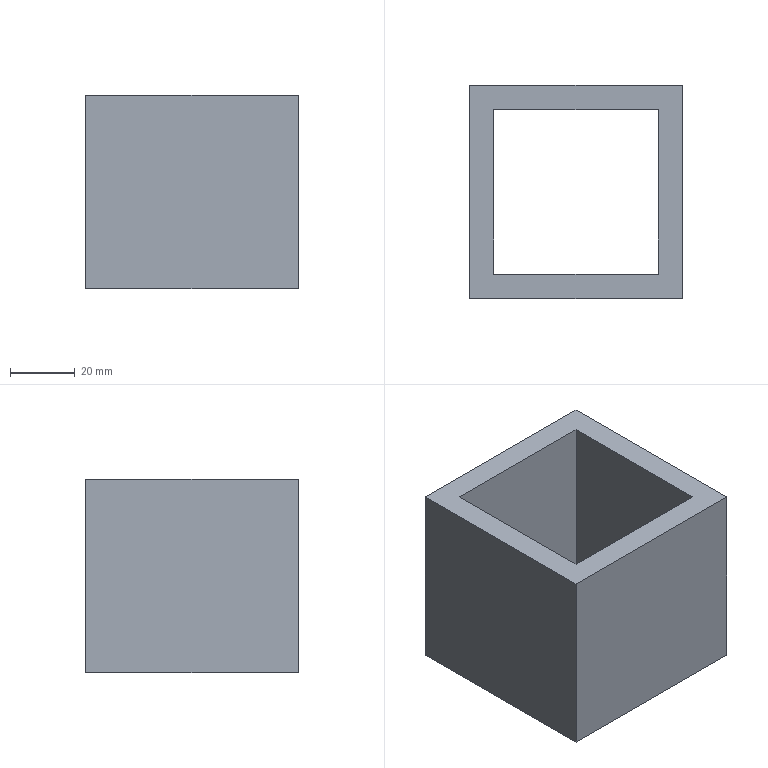Part | SolidWorks | features Extrusion 1 | 1 solid | 10 faces | box 66 x 66 x 60 mm | volume 105300 mm3 | plane 10
STEP:
#1=CARTESIAN_POINT('',(-33.,33.,30.));
#2=VERTEX_POINT('',#1);
#3=CARTESIAN_POINT('',(-33.,-33.,30.));
#4=VERTEX_POINT('',#3);
#5=CARTESIAN_POINT('',(-33.,33.,30.));
#6=DIRECTION('',(0.,-1.,0.));
#7=VECTOR('',#6,1000.);
#8=LINE('',#5,#7);
#9=EDGE_CURVE('',#2,#4,#8,.T.);
#10=ORIENTED_EDGE('',*,*,#9,.F.);
#11=CARTESIAN_POINT('',(-33.,33.,-30.));
#12=VERTEX_POINT('',#11);
#13=CARTESIAN_POINT('',(-33.,33.,-30.));
#14=DIRECTION('',(0.,0.,1.));
#15=VECTOR('',#14,1000.);
#16=LINE('',#13,#15);
#17=EDGE_CURVE('',#12,#2,#16,.T.);
#18=ORIENTED_EDGE('',*,*,#17,.F.);
#19=CARTESIAN_POINT('',(-33.,-33.,-30.));
#20=VERTEX_POINT('',#19);
#21=CARTESIAN_POINT('',(-33.,33.,-30.));
#22=DIRECTION('',(0.,-1.,0.));
#23=VECTOR('',#22,1000.);
#24=LINE('',#21,#23);
#25=EDGE_CURVE('',#12,#20,#24,.T.);
#26=ORIENTED_EDGE('',*,*,#25,.T.);
#27=CARTESIAN_POINT('',(-33.,-33.,-30.));
#28=DIRECTION('',(0.,0.,1.));
#29=VECTOR('',#28,1000.);
#30=LINE('',#27,#29);
#31=EDGE_CURVE('',#20,#4,#30,.T.);
#32=ORIENTED_EDGE('',*,*,#31,.T.);
#33=EDGE_LOOP('',(#10,#18,#26,#32));
#34=FACE_OUTER_BOUND('',#33,.T.);
#35=CARTESIAN_POINT('',(-33.,33.,-30.));
#36=DIRECTION('',(-1.,0.,0.));
#37=DIRECTION('',(0.,0.,1.));
#38=AXIS2_PLACEMENT_3D('',#35,#36,#37);
#39=PLANE('',#38);
#40=ADVANCED_FACE('',(#34),#39,.T.);
#41=CARTESIAN_POINT('',(33.,33.,30.));
#42=VERTEX_POINT('',#41);
#43=CARTESIAN_POINT('',(33.,33.,30.));
#44=DIRECTION('',(-1.,0.,0.));
#45=VECTOR('',#44,1000.);
#46=LINE('',#43,#45);
#47=EDGE_CURVE('',#42,#2,#46,.T.);
#48=ORIENTED_EDGE('',*,*,#47,.F.);
#49=CARTESIAN_POINT('',(33.,33.,-30.));
#50=VERTEX_POINT('',#49);
#51=CARTESIAN_POINT('',(33.,33.,-30.));
#52=DIRECTION('',(0.,0.,1.));
#53=VECTOR('',#52,1000.);
#54=LINE('',#51,#53);
#55=EDGE_CURVE('',#50,#42,#54,.T.);
#56=ORIENTED_EDGE('',*,*,#55,.F.);
#57=CARTESIAN_POINT('',(33.,33.,-30.));
#58=DIRECTION('',(-1.,0.,0.));
#59=VECTOR('',#58,1000.);
#60=LINE('',#57,#59);
#61=EDGE_CURVE('',#50,#12,#60,.T.);
#62=ORIENTED_EDGE('',*,*,#61,.T.);
#63=ORIENTED_EDGE('',*,*,#17,.T.);
#64=EDGE_LOOP('',(#48,#56,#62,#63));
#65=FACE_OUTER_BOUND('',#64,.T.);
#66=CARTESIAN_POINT('',(33.,33.,-30.));
#67=DIRECTION('',(0.,1.,0.));
#68=DIRECTION('',(0.,0.,1.));
#69=AXIS2_PLACEMENT_3D('',#66,#67,#68);
#70=PLANE('',#69);
#71=ADVANCED_FACE('',(#65),#70,.T.);
#72=CARTESIAN_POINT('',(33.,-33.,30.));
#73=VERTEX_POINT('',#72);
#74=CARTESIAN_POINT('',(33.,-33.,30.));
#75=DIRECTION('',(0.,1.,0.));
#76=VECTOR('',#75,1000.);
#77=LINE('',#74,#76);
#78=EDGE_CURVE('',#73,#42,#77,.T.);
#79=ORIENTED_EDGE('',*,*,#78,.F.);
#80=CARTESIAN_POINT('',(33.,-33.,-30.));
#81=VERTEX_POINT('',#80);
#82=CARTESIAN_POINT('',(33.,-33.,-30.));
#83=DIRECTION('',(0.,0.,1.));
#84=VECTOR('',#83,1000.);
#85=LINE('',#82,#84);
#86=EDGE_CURVE('',#81,#73,#85,.T.);
#87=ORIENTED_EDGE('',*,*,#86,.F.);
#88=CARTESIAN_POINT('',(33.,-33.,-30.));
#89=DIRECTION('',(0.,1.,0.));
#90=VECTOR('',#89,1000.);
#91=LINE('',#88,#90);
#92=EDGE_CURVE('',#81,#50,#91,.T.);
#93=ORIENTED_EDGE('',*,*,#92,.T.);
#94=ORIENTED_EDGE('',*,*,#55,.T.);
#95=EDGE_LOOP('',(#79,#87,#93,#94));
#96=FACE_OUTER_BOUND('',#95,.T.);
#97=CARTESIAN_POINT('',(33.,-33.,-30.));
#98=DIRECTION('',(1.,0.,0.));
#99=DIRECTION('',(0.,0.,-1.));
#100=AXIS2_PLACEMENT_3D('',#97,#98,#99);
#101=PLANE('',#100);
#102=ADVANCED_FACE('',(#96),#101,.T.);
#103=CARTESIAN_POINT('',(-33.,-33.,30.));
#104=DIRECTION('',(1.,0.,0.));
#105=VECTOR('',#104,1000.);
#106=LINE('',#103,#105);
#107=EDGE_CURVE('',#4,#73,#106,.T.);
#108=ORIENTED_EDGE('',*,*,#107,.F.);
#109=ORIENTED_EDGE('',*,*,#31,.F.);
#110=CARTESIAN_POINT('',(-33.,-33.,-30.));
#111=DIRECTION('',(1.,0.,0.));
#112=VECTOR('',#111,1000.);
#113=LINE('',#110,#112);
#114=EDGE_CURVE('',#20,#81,#113,.T.);
#115=ORIENTED_EDGE('',*,*,#114,.T.);
#116=ORIENTED_EDGE('',*,*,#86,.T.);
#117=EDGE_LOOP('',(#108,#109,#115,#116));
#118=FACE_OUTER_BOUND('',#117,.T.);
#119=CARTESIAN_POINT('',(-33.,-33.,-30.));
#120=DIRECTION('',(0.,-1.,0.));
#121=DIRECTION('',(0.,0.,-1.));
#122=AXIS2_PLACEMENT_3D('',#119,#120,#121);
#123=PLANE('',#122);
#124=ADVANCED_FACE('',(#118),#123,.T.);
#125=CARTESIAN_POINT('',(25.5,25.5,-30.));
#126=VERTEX_POINT('',#125);
#127=CARTESIAN_POINT('',(-25.5,25.5,-30.));
#128=VERTEX_POINT('',#127);
#129=CARTESIAN_POINT('',(25.5,25.5,-30.));
#130=DIRECTION('',(-1.,0.,0.));
#131=VECTOR('',#130,1000.);
#132=LINE('',#129,#131);
#133=EDGE_CURVE('',#126,#128,#132,.T.);
#134=ORIENTED_EDGE('',*,*,#133,.T.);
#135=CARTESIAN_POINT('',(-25.5,-25.5,-30.));
#136=VERTEX_POINT('',#135);
#137=CARTESIAN_POINT('',(-25.5,25.5,-30.));
#138=DIRECTION('',(0.,-1.,0.));
#139=VECTOR('',#138,1000.);
#140=LINE('',#137,#139);
#141=EDGE_CURVE('',#128,#136,#140,.T.);
#142=ORIENTED_EDGE('',*,*,#141,.T.);
#143=CARTESIAN_POINT('',(25.5,-25.5,-30.));
#144=VERTEX_POINT('',#143);
#145=CARTESIAN_POINT('',(-25.5,-25.5,-30.));
#146=DIRECTION('',(1.,0.,0.));
#147=VECTOR('',#146,1000.);
#148=LINE('',#145,#147);
#149=EDGE_CURVE('',#136,#144,#148,.T.);
#150=ORIENTED_EDGE('',*,*,#149,.T.);
#151=CARTESIAN_POINT('',(25.5,-25.5,-30.));
#152=DIRECTION('',(0.,1.,0.));
#153=VECTOR('',#152,1000.);
#154=LINE('',#151,#153);
#155=EDGE_CURVE('',#144,#126,#154,.T.);
#156=ORIENTED_EDGE('',*,*,#155,.T.);
#157=EDGE_LOOP('',(#134,#142,#150,#156));
#158=FACE_BOUND('',#157,.T.);
#159=ORIENTED_EDGE('',*,*,#25,.F.);
#160=ORIENTED_EDGE('',*,*,#61,.F.);
#161=ORIENTED_EDGE('',*,*,#92,.F.);
#162=ORIENTED_EDGE('',*,*,#114,.F.);
#163=EDGE_LOOP('',(#159,#160,#161,#162));
#164=FACE_OUTER_BOUND('',#163,.T.);
#165=CARTESIAN_POINT('',(0.,0.,-30.));
#166=DIRECTION('',(0.,0.,1.));
#167=DIRECTION('',(1.,0.,0.));
#168=AXIS2_PLACEMENT_3D('',#165,#166,#167);
#169=PLANE('',#168);
#170=ADVANCED_FACE('',(#158,#164),#169,.F.);
#171=CARTESIAN_POINT('',(-25.5,25.5,30.));
#172=VERTEX_POINT('',#171);
#173=CARTESIAN_POINT('',(-25.5,-25.5,30.));
#174=VERTEX_POINT('',#173);
#175=CARTESIAN_POINT('',(-25.5,25.5,30.));
#176=DIRECTION('',(0.,-1.,0.));
#177=VECTOR('',#176,1000.);
#178=LINE('',#175,#177);
#179=EDGE_CURVE('',#172,#174,#178,.T.);
#180=ORIENTED_EDGE('',*,*,#179,.F.);
#181=CARTESIAN_POINT('',(25.5,25.5,30.));
#182=VERTEX_POINT('',#181);
#183=CARTESIAN_POINT('',(25.5,25.5,30.));
#184=DIRECTION('',(-1.,0.,0.));
#185=VECTOR('',#184,1000.);
#186=LINE('',#183,#185);
#187=EDGE_CURVE('',#182,#172,#186,.T.);
#188=ORIENTED_EDGE('',*,*,#187,.F.);
#189=CARTESIAN_POINT('',(25.5,-25.5,30.));
#190=VERTEX_POINT('',#189);
#191=CARTESIAN_POINT('',(25.5,-25.5,30.));
#192=DIRECTION('',(0.,1.,0.));
#193=VECTOR('',#192,1000.);
#194=LINE('',#191,#193);
#195=EDGE_CURVE('',#190,#182,#194,.T.);
#196=ORIENTED_EDGE('',*,*,#195,.F.);
#197=CARTESIAN_POINT('',(-25.5,-25.5,30.));
#198=DIRECTION('',(1.,0.,0.));
#199=VECTOR('',#198,1000.);
#200=LINE('',#197,#199);
#201=EDGE_CURVE('',#174,#190,#200,.T.);
#202=ORIENTED_EDGE('',*,*,#201,.F.);
#203=EDGE_LOOP('',(#180,#188,#196,#202));
#204=FACE_BOUND('',#203,.T.);
#205=ORIENTED_EDGE('',*,*,#9,.T.);
#206=ORIENTED_EDGE('',*,*,#107,.T.);
#207=ORIENTED_EDGE('',*,*,#78,.T.);
#208=ORIENTED_EDGE('',*,*,#47,.T.);
#209=EDGE_LOOP('',(#205,#206,#207,#208));
#210=FACE_OUTER_BOUND('',#209,.T.);
#211=CARTESIAN_POINT('',(0.,0.,30.));
#212=DIRECTION('',(0.,0.,1.));
#213=DIRECTION('',(1.,0.,0.));
#214=AXIS2_PLACEMENT_3D('',#211,#212,#213);
#215=PLANE('',#214);
#216=ADVANCED_FACE('',(#204,#210),#215,.T.);
#217=ORIENTED_EDGE('',*,*,#179,.T.);
#218=CARTESIAN_POINT('',(-25.5,-25.5,-30.));
#219=DIRECTION('',(0.,0.,1.));
#220=VECTOR('',#219,1000.);
#221=LINE('',#218,#220);
#222=EDGE_CURVE('',#136,#174,#221,.T.);
#223=ORIENTED_EDGE('',*,*,#222,.F.);
#224=ORIENTED_EDGE('',*,*,#141,.F.);
#225=CARTESIAN_POINT('',(-25.5,25.5,-30.));
#226=DIRECTION('',(0.,0.,1.));
#227=VECTOR('',#226,1000.);
#228=LINE('',#225,#227);
#229=EDGE_CURVE('',#128,#172,#228,.T.);
#230=ORIENTED_EDGE('',*,*,#229,.T.);
#231=EDGE_LOOP('',(#217,#223,#224,#230));
#232=FACE_OUTER_BOUND('',#231,.T.);
#233=CARTESIAN_POINT('',(-25.5,25.5,-30.));
#234=DIRECTION('',(-1.,0.,0.));
#235=DIRECTION('',(0.,0.,1.));
#236=AXIS2_PLACEMENT_3D('',#233,#234,#235);
#237=PLANE('',#236);
#238=ADVANCED_FACE('',(#232),#237,.F.);
#239=ORIENTED_EDGE('',*,*,#187,.T.);
#240=ORIENTED_EDGE('',*,*,#229,.F.);
#241=ORIENTED_EDGE('',*,*,#133,.F.);
#242=CARTESIAN_POINT('',(25.5,25.5,-30.));
#243=DIRECTION('',(0.,0.,1.));
#244=VECTOR('',#243,1000.);
#245=LINE('',#242,#244);
#246=EDGE_CURVE('',#126,#182,#245,.T.);
#247=ORIENTED_EDGE('',*,*,#246,.T.);
#248=EDGE_LOOP('',(#239,#240,#241,#247));
#249=FACE_OUTER_BOUND('',#248,.T.);
#250=CARTESIAN_POINT('',(25.5,25.5,-30.));
#251=DIRECTION('',(0.,1.,0.));
#252=DIRECTION('',(0.,0.,1.));
#253=AXIS2_PLACEMENT_3D('',#250,#251,#252);
#254=PLANE('',#253);
#255=ADVANCED_FACE('',(#249),#254,.F.);
#256=ORIENTED_EDGE('',*,*,#195,.T.);
#257=ORIENTED_EDGE('',*,*,#246,.F.);
#258=ORIENTED_EDGE('',*,*,#155,.F.);
#259=CARTESIAN_POINT('',(25.5,-25.5,-30.));
#260=DIRECTION('',(0.,0.,1.));
#261=VECTOR('',#260,1000.);
#262=LINE('',#259,#261);
#263=EDGE_CURVE('',#144,#190,#262,.T.);
#264=ORIENTED_EDGE('',*,*,#263,.T.);
#265=EDGE_LOOP('',(#256,#257,#258,#264));
#266=FACE_OUTER_BOUND('',#265,.T.);
#267=CARTESIAN_POINT('',(25.5,-25.5,-30.));
#268=DIRECTION('',(1.,0.,0.));
#269=DIRECTION('',(0.,0.,-1.));
#270=AXIS2_PLACEMENT_3D('',#267,#268,#269);
#271=PLANE('',#270);
#272=ADVANCED_FACE('',(#266),#271,.F.);
#273=ORIENTED_EDGE('',*,*,#201,.T.);
#274=ORIENTED_EDGE('',*,*,#263,.F.);
#275=ORIENTED_EDGE('',*,*,#149,.F.);
#276=ORIENTED_EDGE('',*,*,#222,.T.);
#277=EDGE_LOOP('',(#273,#274,#275,#276));
#278=FACE_OUTER_BOUND('',#277,.T.);
#279=CARTESIAN_POINT('',(-25.5,-25.5,-30.));
#280=DIRECTION('',(0.,-1.,0.));
#281=DIRECTION('',(0.,0.,-1.));
#282=AXIS2_PLACEMENT_3D('',#279,#280,#281);
#283=PLANE('',#282);
#284=ADVANCED_FACE('',(#278),#283,.F.);
#285=CLOSED_SHELL('',(#40,#71,#102,#124,#170,#216,#238,#255,#272,#284));
#286=MANIFOLD_SOLID_BREP('',#285);
#287=CARTESIAN_POINT('',(0.,0.,0.));
#288=DIRECTION('',(0.,0.,1.));
#289=DIRECTION('',(1.,0.,0.));
#290=AXIS2_PLACEMENT_3D('',#287,#288,#289);
#291=(LENGTH_UNIT()NAMED_UNIT(*)SI_UNIT(.MILLI.,.METRE.));
#292=UNCERTAINTY_MEASURE_WITH_UNIT(LENGTH_MEASURE(0.00001),#291,'','');
#293=(NAMED_UNIT(*)PLANE_ANGLE_UNIT()SI_UNIT($,.RADIAN.));
#294=(NAMED_UNIT(*)SI_UNIT($,.STERADIAN.)SOLID_ANGLE_UNIT());
#295=(GEOMETRIC_REPRESENTATION_CONTEXT(3)GLOBAL_UNCERTAINTY_ASSIGNED_CONTEXT((#292))GLOBAL_UNIT_ASSIGNED_CONTEXT((#291,#293,#294))REPRESENTATION_CONTEXT('',''));
#296=ADVANCED_BREP_SHAPE_REPRESENTATION('',(#286,#290),#295);